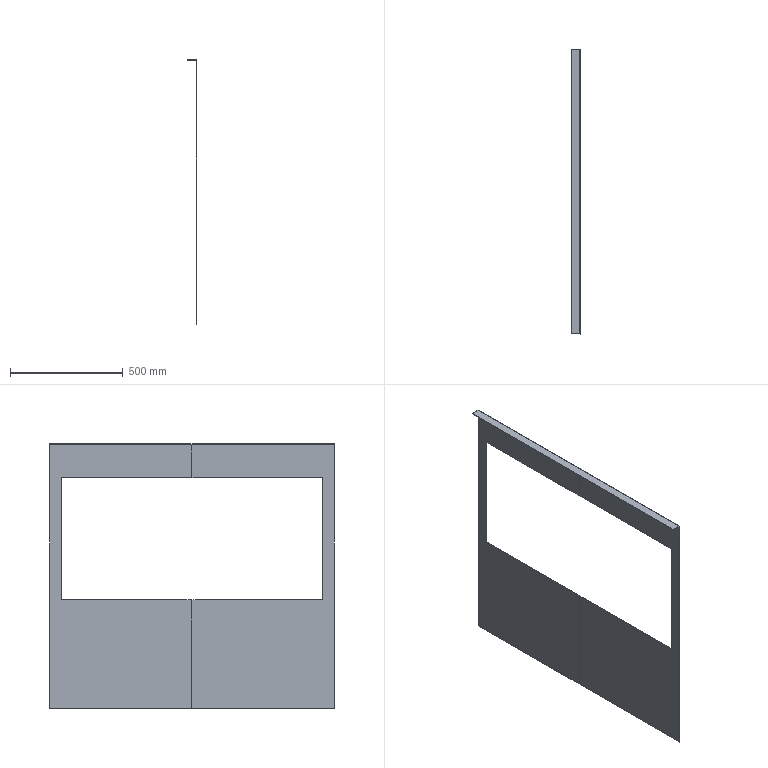Part | NX | features BREP 1 | 1 solid | 23 faces | box 42 x 1258 x 1171 mm | volume 1789977 mm3 | plane 20 | cylinder 3 | commonest cylinder face diameters 6 x2 10 x1
STEP:
#1=CARTESIAN_POINT('',(2104.579,0.000000001,74.));
#2=VERTEX_POINT('',#1);
#3=CARTESIAN_POINT('',(2104.579,0.,553.577));
#4=VERTEX_POINT('',#3);
#5=CARTESIAN_POINT('',(2104.579,-0.000000001,313.789));
#6=DIRECTION('',(0.,0.,1.));
#7=VECTOR('',#6,1000.);
#8=LINE('',#5,#7);
#9=EDGE_CURVE('',#2,#4,#8,.T.);
#10=ORIENTED_EDGE('',*,*,#9,.F.);
#11=CARTESIAN_POINT('',(2104.579,-629.17,74.));
#12=VERTEX_POINT('',#11);
#13=CARTESIAN_POINT('',(2104.579,-314.585,74.));
#14=DIRECTION('',(0.,-1.,0.));
#15=VECTOR('',#14,1000.);
#16=LINE('',#13,#15);
#17=EDGE_CURVE('',#2,#12,#16,.T.);
#18=ORIENTED_EDGE('',*,*,#17,.T.);
#19=CARTESIAN_POINT('',(2104.579,-629.17,1239.934));
#20=VERTEX_POINT('',#19);
#21=CARTESIAN_POINT('',(2104.579,-629.17,656.967));
#22=DIRECTION('',(0.,0.,1.));
#23=VECTOR('',#22,1000.);
#24=LINE('',#21,#23);
#25=EDGE_CURVE('',#12,#20,#24,.T.);
#26=ORIENTED_EDGE('',*,*,#25,.T.);
#27=CARTESIAN_POINT('',(2104.579,0.,1239.934));
#28=VERTEX_POINT('',#27);
#29=CARTESIAN_POINT('',(2104.579,0.,1239.934));
#30=DIRECTION('',(0.,-1.,0.));
#31=VECTOR('',#30,1000.);
#32=LINE('',#29,#31);
#33=EDGE_CURVE('',#28,#20,#32,.T.);
#34=ORIENTED_EDGE('',*,*,#33,.F.);
#35=CARTESIAN_POINT('',(2104.579,0.000000001,1094.538));
#36=VERTEX_POINT('',#35);
#37=CARTESIAN_POINT('',(2104.579,-0.000000001,1167.236));
#38=DIRECTION('',(0.,0.,1.));
#39=VECTOR('',#38,1000.);
#40=LINE('',#37,#39);
#41=EDGE_CURVE('',#36,#28,#40,.T.);
#42=ORIENTED_EDGE('',*,*,#41,.F.);
#43=CARTESIAN_POINT('',(2104.579,-579.171,1094.538));
#44=VERTEX_POINT('',#43);
#45=CARTESIAN_POINT('',(2104.579,-289.585,1094.538));
#46=DIRECTION('',(0.,-1.,0.));
#47=VECTOR('',#46,1000.);
#48=LINE('',#45,#47);
#49=EDGE_CURVE('',#36,#44,#48,.T.);
#50=ORIENTED_EDGE('',*,*,#49,.T.);
#51=CARTESIAN_POINT('',(2104.579,-579.171,553.577));
#52=VERTEX_POINT('',#51);
#53=CARTESIAN_POINT('',(2104.579,-579.171,824.058));
#54=DIRECTION('',(0.,0.,1.));
#55=VECTOR('',#54,1000.);
#56=LINE('',#53,#55);
#57=EDGE_CURVE('',#52,#44,#56,.T.);
#58=ORIENTED_EDGE('',*,*,#57,.F.);
#59=CARTESIAN_POINT('',(2104.579,-21.22,553.577));
#60=VERTEX_POINT('',#59);
#61=CARTESIAN_POINT('',(2104.579,-300.195,553.577));
#62=DIRECTION('',(0.,-1.,0.));
#63=VECTOR('',#62,1000.);
#64=LINE('',#61,#63);
#65=EDGE_CURVE('',#52,#60,#64,.F.);
#66=ORIENTED_EDGE('',*,*,#65,.T.);
#67=CARTESIAN_POINT('',(2104.579,-8.78,553.577));
#68=VERTEX_POINT('',#67);
#69=CARTESIAN_POINT('',(2104.579,-15.,553.577));
#70=DIRECTION('',(0.,-1.,0.));
#71=VECTOR('',#70,1000.);
#72=LINE('',#69,#71);
#73=EDGE_CURVE('',#68,#60,#72,.T.);
#74=ORIENTED_EDGE('',*,*,#73,.F.);
#75=CARTESIAN_POINT('',(2104.579,-4.39,553.577));
#76=DIRECTION('',(0.,1.,0.));
#77=VECTOR('',#76,1000.);
#78=LINE('',#75,#77);
#79=EDGE_CURVE('',#4,#68,#78,.F.);
#80=ORIENTED_EDGE('',*,*,#79,.F.);
#81=EDGE_LOOP('',(#10,#18,#26,#34,#42,#50,#58,#66,#74,#80));
#82=FACE_BOUND('',#81,.T.);
#83=CARTESIAN_POINT('',(2104.579,0.,74.));
#84=DIRECTION('',(-1.,0.,0.));
#85=DIRECTION('',(0.,-1.,0.));
#86=AXIS2_PLACEMENT_3D('',#83,#84,#85);
#87=PLANE('',#86);
#88=ADVANCED_FACE('',(#82),#87,.T.);
#89=CARTESIAN_POINT('',(2104.579,8.78,553.577));
#90=VERTEX_POINT('',#89);
#91=CARTESIAN_POINT('',(2104.579,4.39,553.577));
#92=DIRECTION('',(0.,1.,0.));
#93=VECTOR('',#92,1000.);
#94=LINE('',#91,#93);
#95=EDGE_CURVE('',#4,#90,#94,.T.);
#96=ORIENTED_EDGE('',*,*,#95,.T.);
#97=CARTESIAN_POINT('',(2104.579,579.171,553.577));
#98=VERTEX_POINT('',#97);
#99=CARTESIAN_POINT('',(2104.579,293.975,553.577));
#100=DIRECTION('',(0.,1.,0.));
#101=VECTOR('',#100,1000.);
#102=LINE('',#99,#101);
#103=EDGE_CURVE('',#90,#98,#102,.T.);
#104=ORIENTED_EDGE('',*,*,#103,.T.);
#105=CARTESIAN_POINT('',(2104.579,579.171,1094.538));
#106=VERTEX_POINT('',#105);
#107=CARTESIAN_POINT('',(2104.579,579.171,824.058));
#108=DIRECTION('',(0.,0.,1.));
#109=VECTOR('',#108,1000.);
#110=LINE('',#107,#109);
#111=EDGE_CURVE('',#98,#106,#110,.T.);
#112=ORIENTED_EDGE('',*,*,#111,.T.);
#113=CARTESIAN_POINT('',(2104.579,289.585,1094.538));
#114=DIRECTION('',(0.,1.,0.));
#115=VECTOR('',#114,1000.);
#116=LINE('',#113,#115);
#117=EDGE_CURVE('',#36,#106,#116,.T.);
#118=ORIENTED_EDGE('',*,*,#117,.F.);
#119=ORIENTED_EDGE('',*,*,#41,.T.);
#120=CARTESIAN_POINT('',(2104.579,629.17,1239.934));
#121=VERTEX_POINT('',#120);
#122=CARTESIAN_POINT('',(2104.579,0.,1239.934));
#123=DIRECTION('',(0.,-1.,0.));
#124=VECTOR('',#123,1000.);
#125=LINE('',#122,#124);
#126=EDGE_CURVE('',#121,#28,#125,.T.);
#127=ORIENTED_EDGE('',*,*,#126,.F.);
#128=CARTESIAN_POINT('',(2104.579,629.17,74.));
#129=VERTEX_POINT('',#128);
#130=CARTESIAN_POINT('',(2104.579,629.17,656.967));
#131=DIRECTION('',(0.,0.,1.));
#132=VECTOR('',#131,1000.);
#133=LINE('',#130,#132);
#134=EDGE_CURVE('',#129,#121,#133,.T.);
#135=ORIENTED_EDGE('',*,*,#134,.F.);
#136=CARTESIAN_POINT('',(2104.579,314.585,74.));
#137=DIRECTION('',(0.,1.,0.));
#138=VECTOR('',#137,1000.);
#139=LINE('',#136,#138);
#140=EDGE_CURVE('',#2,#129,#139,.T.);
#141=ORIENTED_EDGE('',*,*,#140,.F.);
#142=ORIENTED_EDGE('',*,*,#9,.T.);
#143=EDGE_LOOP('',(#96,#104,#112,#118,#119,#127,#135,#141,#142));
#144=FACE_BOUND('',#143,.T.);
#145=CARTESIAN_POINT('',(2104.579,0.,74.));
#146=DIRECTION('',(1.,0.,0.));
#147=DIRECTION('',(0.,1.,0.));
#148=AXIS2_PLACEMENT_3D('',#145,#146,#147);
#149=PLANE('',#148);
#150=ADVANCED_FACE('',(#144),#149,.F.);
#151=CARTESIAN_POINT('',(2106.579,579.171,553.577));
#152=VERTEX_POINT('',#151);
#153=CARTESIAN_POINT('',(2106.579,579.171,1094.538));
#154=VERTEX_POINT('',#153);
#155=CARTESIAN_POINT('',(2106.579,579.171,824.058));
#156=DIRECTION('',(0.,0.,1.));
#157=VECTOR('',#156,1000.);
#158=LINE('',#155,#157);
#159=EDGE_CURVE('',#152,#154,#158,.T.);
#160=ORIENTED_EDGE('',*,*,#159,.T.);
#161=CARTESIAN_POINT('',(2105.579,579.171,1094.538));
#162=DIRECTION('',(1.,-0.000000002,0.));
#163=VECTOR('',#162,1000.);
#164=LINE('',#161,#163);
#165=EDGE_CURVE('',#106,#154,#164,.T.);
#166=ORIENTED_EDGE('',*,*,#165,.F.);
#167=ORIENTED_EDGE('',*,*,#111,.F.);
#168=CARTESIAN_POINT('',(2105.579,579.171,553.577));
#169=DIRECTION('',(1.,0.,0.));
#170=VECTOR('',#169,1000.);
#171=LINE('',#168,#170);
#172=EDGE_CURVE('',#98,#152,#171,.T.);
#173=ORIENTED_EDGE('',*,*,#172,.T.);
#174=EDGE_LOOP('',(#160,#166,#167,#173));
#175=FACE_BOUND('',#174,.T.);
#176=CARTESIAN_POINT('',(2106.579,579.171,553.577));
#177=DIRECTION('',(0.,1.,0.));
#178=DIRECTION('',(0.,0.,1.));
#179=AXIS2_PLACEMENT_3D('',#176,#177,#178);
#180=PLANE('',#179);
#181=ADVANCED_FACE('',(#175),#180,.F.);
#182=CARTESIAN_POINT('',(2106.579,0.,1094.538));
#183=VERTEX_POINT('',#182);
#184=CARTESIAN_POINT('',(2106.579,289.585,1094.538));
#185=DIRECTION('',(0.,1.,0.));
#186=VECTOR('',#185,1000.);
#187=LINE('',#184,#186);
#188=EDGE_CURVE('',#183,#154,#187,.T.);
#189=ORIENTED_EDGE('',*,*,#188,.F.);
#190=CARTESIAN_POINT('',(2105.579,0.,1094.538));
#191=DIRECTION('',(-1.,0.,0.));
#192=VECTOR('',#191,1000.);
#193=LINE('',#190,#192);
#194=EDGE_CURVE('',#183,#36,#193,.T.);
#195=ORIENTED_EDGE('',*,*,#194,.T.);
#196=ORIENTED_EDGE('',*,*,#117,.T.);
#197=ORIENTED_EDGE('',*,*,#165,.T.);
#198=EDGE_LOOP('',(#189,#195,#196,#197));
#199=FACE_BOUND('',#198,.T.);
#200=CARTESIAN_POINT('',(2106.579,579.171,1094.538));
#201=DIRECTION('',(0.,0.,1.));
#202=DIRECTION('',(0.,-1.,0.));
#203=AXIS2_PLACEMENT_3D('',#200,#201,#202);
#204=PLANE('',#203);
#205=ADVANCED_FACE('',(#199),#204,.F.);
#206=CARTESIAN_POINT('',(2106.579,0.,74.));
#207=VERTEX_POINT('',#206);
#208=CARTESIAN_POINT('',(2106.579,629.17,74.));
#209=VERTEX_POINT('',#208);
#210=CARTESIAN_POINT('',(2106.579,314.585,74.));
#211=DIRECTION('',(0.,1.,0.));
#212=VECTOR('',#211,1000.);
#213=LINE('',#210,#212);
#214=EDGE_CURVE('',#207,#209,#213,.T.);
#215=ORIENTED_EDGE('',*,*,#214,.F.);
#216=CARTESIAN_POINT('',(2105.579,0.,74.));
#217=DIRECTION('',(-1.,0.,0.));
#218=VECTOR('',#217,1000.);
#219=LINE('',#216,#218);
#220=EDGE_CURVE('',#207,#2,#219,.T.);
#221=ORIENTED_EDGE('',*,*,#220,.T.);
#222=ORIENTED_EDGE('',*,*,#140,.T.);
#223=CARTESIAN_POINT('',(2105.579,629.17,74.));
#224=DIRECTION('',(1.,0.,0.));
#225=VECTOR('',#224,1000.);
#226=LINE('',#223,#225);
#227=EDGE_CURVE('',#129,#209,#226,.T.);
#228=ORIENTED_EDGE('',*,*,#227,.T.);
#229=EDGE_LOOP('',(#215,#221,#222,#228));
#230=FACE_BOUND('',#229,.T.);
#231=CARTESIAN_POINT('',(2106.579,314.585,74.));
#232=DIRECTION('',(0.,0.,-1.));
#233=DIRECTION('',(1.,0.,0.));
#234=AXIS2_PLACEMENT_3D('',#231,#232,#233);
#235=PLANE('',#234);
#236=ADVANCED_FACE('',(#230),#235,.T.);
#237=CARTESIAN_POINT('',(2106.579,-629.17,74.));
#238=VERTEX_POINT('',#237);
#239=CARTESIAN_POINT('',(2105.579,-629.17,74.));
#240=DIRECTION('',(-1.,0.,0.));
#241=VECTOR('',#240,1000.);
#242=LINE('',#239,#241);
#243=EDGE_CURVE('',#238,#12,#242,.T.);
#244=ORIENTED_EDGE('',*,*,#243,.T.);
#245=ORIENTED_EDGE('',*,*,#17,.F.);
#246=ORIENTED_EDGE('',*,*,#220,.F.);
#247=CARTESIAN_POINT('',(2106.579,-314.585,74.));
#248=DIRECTION('',(0.,-1.,0.));
#249=VECTOR('',#248,1000.);
#250=LINE('',#247,#249);
#251=EDGE_CURVE('',#207,#238,#250,.T.);
#252=ORIENTED_EDGE('',*,*,#251,.T.);
#253=EDGE_LOOP('',(#244,#245,#246,#252));
#254=FACE_BOUND('',#253,.T.);
#255=CARTESIAN_POINT('',(2106.579,0.,74.));
#256=DIRECTION('',(0.,0.,-1.));
#257=DIRECTION('',(0.,-1.,0.));
#258=AXIS2_PLACEMENT_3D('',#255,#256,#257);
#259=PLANE('',#258);
#260=ADVANCED_FACE('',(#254),#259,.T.);
#261=CARTESIAN_POINT('',(2106.579,-579.171,1094.538));
#262=VERTEX_POINT('',#261);
#263=CARTESIAN_POINT('',(2105.579,-579.171,1094.538));
#264=DIRECTION('',(-1.,0.,0.));
#265=VECTOR('',#264,1000.);
#266=LINE('',#263,#265);
#267=EDGE_CURVE('',#262,#44,#266,.T.);
#268=ORIENTED_EDGE('',*,*,#267,.T.);
#269=ORIENTED_EDGE('',*,*,#49,.F.);
#270=ORIENTED_EDGE('',*,*,#194,.F.);
#271=CARTESIAN_POINT('',(2106.579,-289.585,1094.538));
#272=DIRECTION('',(0.,-1.,0.));
#273=VECTOR('',#272,1000.);
#274=LINE('',#271,#273);
#275=EDGE_CURVE('',#183,#262,#274,.T.);
#276=ORIENTED_EDGE('',*,*,#275,.T.);
#277=EDGE_LOOP('',(#268,#269,#270,#276));
#278=FACE_BOUND('',#277,.T.);
#279=CARTESIAN_POINT('',(2106.579,-579.171,1094.538));
#280=DIRECTION('',(0.,0.,1.));
#281=DIRECTION('',(0.,1.,0.));
#282=AXIS2_PLACEMENT_3D('',#279,#280,#281);
#283=PLANE('',#282);
#284=ADVANCED_FACE('',(#278),#283,.F.);
#285=CARTESIAN_POINT('',(2106.579,-579.171,553.577));
#286=VERTEX_POINT('',#285);
#287=CARTESIAN_POINT('',(2105.579,-579.171,553.577));
#288=DIRECTION('',(-1.,0.,0.));
#289=VECTOR('',#288,1000.);
#290=LINE('',#287,#289);
#291=EDGE_CURVE('',#286,#52,#290,.T.);
#292=ORIENTED_EDGE('',*,*,#291,.T.);
#293=ORIENTED_EDGE('',*,*,#57,.T.);
#294=ORIENTED_EDGE('',*,*,#267,.F.);
#295=CARTESIAN_POINT('',(2106.579,-579.171,824.058));
#296=DIRECTION('',(0.,0.,1.));
#297=VECTOR('',#296,1000.);
#298=LINE('',#295,#297);
#299=EDGE_CURVE('',#286,#262,#298,.T.);
#300=ORIENTED_EDGE('',*,*,#299,.F.);
#301=EDGE_LOOP('',(#292,#293,#294,#300));
#302=FACE_BOUND('',#301,.T.);
#303=CARTESIAN_POINT('',(2106.579,-579.171,553.577));
#304=DIRECTION('',(0.,-1.,0.));
#305=DIRECTION('',(0.,0.,1.));
#306=AXIS2_PLACEMENT_3D('',#303,#304,#305);
#307=PLANE('',#306);
#308=ADVANCED_FACE('',(#302),#307,.F.);
#309=ORIENTED_EDGE('',*,*,#73,.T.);
#310=ORIENTED_EDGE('',*,*,#65,.F.);
#311=ORIENTED_EDGE('',*,*,#291,.F.);
#312=CARTESIAN_POINT('',(2106.579,-21.22,553.577));
#313=VERTEX_POINT('',#312);
#314=CARTESIAN_POINT('',(2106.579,-300.195,553.577));
#315=DIRECTION('',(0.,-1.,0.));
#316=VECTOR('',#315,1000.);
#317=LINE('',#314,#316);
#318=EDGE_CURVE('',#313,#286,#317,.T.);
#319=ORIENTED_EDGE('',*,*,#318,.F.);
#320=CARTESIAN_POINT('',(2106.579,-8.78,553.577));
#321=VERTEX_POINT('',#320);
#322=CARTESIAN_POINT('',(2106.579,-15.,553.577));
#323=DIRECTION('',(0.,-1.,0.));
#324=VECTOR('',#323,1000.);
#325=LINE('',#322,#324);
#326=EDGE_CURVE('',#321,#313,#325,.T.);
#327=ORIENTED_EDGE('',*,*,#326,.F.);
#328=CARTESIAN_POINT('',(2106.579,0.,553.577));
#329=VERTEX_POINT('',#328);
#330=CARTESIAN_POINT('',(2106.579,-4.39,553.577));
#331=DIRECTION('',(0.,-1.,0.));
#332=VECTOR('',#331,1000.);
#333=LINE('',#330,#332);
#334=EDGE_CURVE('',#329,#321,#333,.T.);
#335=ORIENTED_EDGE('',*,*,#334,.F.);
#336=CARTESIAN_POINT('',(2106.579,8.78,553.577));
#337=VERTEX_POINT('',#336);
#338=CARTESIAN_POINT('',(2106.579,4.39,553.577));
#339=DIRECTION('',(0.,1.,0.));
#340=VECTOR('',#339,1000.);
#341=LINE('',#338,#340);
#342=EDGE_CURVE('',#329,#337,#341,.T.);
#343=ORIENTED_EDGE('',*,*,#342,.T.);
#344=CARTESIAN_POINT('',(2106.579,293.975,553.577));
#345=DIRECTION('',(0.,1.,0.));
#346=VECTOR('',#345,1000.);
#347=LINE('',#344,#346);
#348=EDGE_CURVE('',#337,#152,#347,.T.);
#349=ORIENTED_EDGE('',*,*,#348,.T.);
#350=ORIENTED_EDGE('',*,*,#172,.F.);
#351=ORIENTED_EDGE('',*,*,#103,.F.);
#352=ORIENTED_EDGE('',*,*,#95,.F.);
#353=ORIENTED_EDGE('',*,*,#79,.T.);
#354=EDGE_LOOP('',(#309,#310,#311,#319,#327,#335,#343,#349,#350,#351,#352,#353));
#355=FACE_BOUND('',#354,.T.);
#356=CARTESIAN_POINT('',(2106.579,8.78,553.577));
#357=DIRECTION('',(0.,0.,-1.));
#358=DIRECTION('',(0.,1.,0.));
#359=AXIS2_PLACEMENT_3D('',#356,#357,#358);
#360=PLANE('',#359);
#361=ADVANCED_FACE('',(#355),#360,.F.);
#362=CARTESIAN_POINT('',(2106.579,-629.17,1239.934));
#363=VERTEX_POINT('',#362);
#364=CARTESIAN_POINT('',(2105.579,-629.17,1239.934));
#365=DIRECTION('',(1.,0.,0.));
#366=VECTOR('',#365,1000.);
#367=LINE('',#364,#366);
#368=EDGE_CURVE('',#20,#363,#367,.T.);
#369=ORIENTED_EDGE('',*,*,#368,.F.);
#370=ORIENTED_EDGE('',*,*,#25,.F.);
#371=ORIENTED_EDGE('',*,*,#243,.F.);
#372=CARTESIAN_POINT('',(2106.579,-629.17,656.967));
#373=DIRECTION('',(0.,0.,1.));
#374=VECTOR('',#373,1000.);
#375=LINE('',#372,#374);
#376=EDGE_CURVE('',#238,#363,#375,.T.);
#377=ORIENTED_EDGE('',*,*,#376,.T.);
#378=EDGE_LOOP('',(#369,#370,#371,#377));
#379=FACE_BOUND('',#378,.T.);
#380=CARTESIAN_POINT('',(2106.579,-629.17,74.));
#381=DIRECTION('',(0.,-1.,0.));
#382=DIRECTION('',(0.,0.,1.));
#383=AXIS2_PLACEMENT_3D('',#380,#381,#382);
#384=PLANE('',#383);
#385=ADVANCED_FACE('',(#379),#384,.T.);
#386=CARTESIAN_POINT('',(2103.7,629.17,1242.055));
#387=VERTEX_POINT('',#386);
#388=CARTESIAN_POINT('',(2101.579,629.17,1239.934));
#389=DIRECTION('',(0.,-1.,0.));
#390=DIRECTION('',(1.,0.,0.));
#391=AXIS2_PLACEMENT_3D('',#388,#389,#390);
#392=CIRCLE('',#391,3.);
#393=EDGE_CURVE('',#121,#387,#392,.T.);
#394=ORIENTED_EDGE('',*,*,#393,.F.);
#395=ORIENTED_EDGE('',*,*,#126,.T.);
#396=ORIENTED_EDGE('',*,*,#33,.T.);
#397=CARTESIAN_POINT('',(2103.7,-629.17,1242.055));
#398=VERTEX_POINT('',#397);
#399=CARTESIAN_POINT('',(2101.579,-629.17,1239.934));
#400=DIRECTION('',(0.,-1.,0.));
#401=DIRECTION('',(1.,0.,0.));
#402=AXIS2_PLACEMENT_3D('',#399,#400,#401);
#403=CIRCLE('',#402,3.);
#404=EDGE_CURVE('',#20,#398,#403,.T.);
#405=ORIENTED_EDGE('',*,*,#404,.T.);
#406=CARTESIAN_POINT('',(2103.7,0.,1242.055));
#407=DIRECTION('',(0.,-1.,0.));
#408=VECTOR('',#407,1000.);
#409=LINE('',#406,#408);
#410=EDGE_CURVE('',#387,#398,#409,.T.);
#411=ORIENTED_EDGE('',*,*,#410,.F.);
#412=EDGE_LOOP('',(#394,#395,#396,#405,#411));
#413=FACE_BOUND('',#412,.T.);
#414=CARTESIAN_POINT('',(2101.579,0.,1239.934));
#415=DIRECTION('',(0.,-1.,0.));
#416=DIRECTION('',(-0.7071,0.,-0.7071));
#417=AXIS2_PLACEMENT_3D('',#414,#415,#416);
#418=CYLINDRICAL_SURFACE('',#417,3.);
#419=ADVANCED_FACE('',(#413),#418,.F.);
#420=CARTESIAN_POINT('',(2106.579,629.17,1239.934));
#421=VERTEX_POINT('',#420);
#422=CARTESIAN_POINT('',(2106.579,629.17,656.967));
#423=DIRECTION('',(0.,0.,1.));
#424=VECTOR('',#423,1000.);
#425=LINE('',#422,#424);
#426=EDGE_CURVE('',#209,#421,#425,.T.);
#427=ORIENTED_EDGE('',*,*,#426,.F.);
#428=ORIENTED_EDGE('',*,*,#227,.F.);
#429=ORIENTED_EDGE('',*,*,#134,.T.);
#430=CARTESIAN_POINT('',(2105.579,629.17,1239.934));
#431=DIRECTION('',(1.,0.,0.));
#432=VECTOR('',#431,1000.);
#433=LINE('',#430,#432);
#434=EDGE_CURVE('',#121,#421,#433,.T.);
#435=ORIENTED_EDGE('',*,*,#434,.T.);
#436=EDGE_LOOP('',(#427,#428,#429,#435));
#437=FACE_BOUND('',#436,.T.);
#438=CARTESIAN_POINT('',(2106.579,629.17,74.));
#439=DIRECTION('',(0.,1.,0.));
#440=DIRECTION('',(0.,0.,1.));
#441=AXIS2_PLACEMENT_3D('',#438,#439,#440);
#442=PLANE('',#441);
#443=ADVANCED_FACE('',(#437),#442,.T.);
#444=CARTESIAN_POINT('',(2106.579,0.,313.789));
#445=DIRECTION('',(0.,0.,1.));
#446=VECTOR('',#445,1000.);
#447=LINE('',#444,#446);
#448=EDGE_CURVE('',#207,#329,#447,.T.);
#449=ORIENTED_EDGE('',*,*,#448,.F.);
#450=ORIENTED_EDGE('',*,*,#214,.T.);
#451=ORIENTED_EDGE('',*,*,#426,.T.);
#452=CARTESIAN_POINT('',(2106.579,0.,1239.934));
#453=VERTEX_POINT('',#452);
#454=CARTESIAN_POINT('',(2106.579,0.,1239.934));
#455=DIRECTION('',(0.,-1.,0.));
#456=VECTOR('',#455,1000.);
#457=LINE('',#454,#456);
#458=EDGE_CURVE('',#421,#453,#457,.T.);
#459=ORIENTED_EDGE('',*,*,#458,.T.);
#460=CARTESIAN_POINT('',(2106.579,0.,1167.236));
#461=DIRECTION('',(0.,0.,1.));
#462=VECTOR('',#461,1000.);
#463=LINE('',#460,#462);
#464=EDGE_CURVE('',#183,#453,#463,.T.);
#465=ORIENTED_EDGE('',*,*,#464,.F.);
#466=ORIENTED_EDGE('',*,*,#188,.T.);
#467=ORIENTED_EDGE('',*,*,#159,.F.);
#468=ORIENTED_EDGE('',*,*,#348,.F.);
#469=ORIENTED_EDGE('',*,*,#342,.F.);
#470=EDGE_LOOP('',(#449,#450,#451,#459,#465,#466,#467,#468,#469));
#471=FACE_BOUND('',#470,.T.);
#472=CARTESIAN_POINT('',(2106.579,-7.184,67.));
#473=DIRECTION('',(1.,0.,0.));
#474=DIRECTION('',(0.,1.,0.));
#475=AXIS2_PLACEMENT_3D('',#472,#473,#474);
#476=PLANE('',#475);
#477=ADVANCED_FACE('',(#471),#476,.T.);
#478=ORIENTED_EDGE('',*,*,#334,.T.);
#479=ORIENTED_EDGE('',*,*,#326,.T.);
#480=ORIENTED_EDGE('',*,*,#318,.T.);
#481=ORIENTED_EDGE('',*,*,#299,.T.);
#482=ORIENTED_EDGE('',*,*,#275,.F.);
#483=ORIENTED_EDGE('',*,*,#464,.T.);
#484=CARTESIAN_POINT('',(2106.579,0.,1239.934));
#485=DIRECTION('',(0.,-1.,0.));
#486=VECTOR('',#485,1000.);
#487=LINE('',#484,#486);
#488=EDGE_CURVE('',#453,#363,#487,.T.);
#489=ORIENTED_EDGE('',*,*,#488,.T.);
#490=ORIENTED_EDGE('',*,*,#376,.F.);
#491=ORIENTED_EDGE('',*,*,#251,.F.);
#492=ORIENTED_EDGE('',*,*,#448,.T.);
#493=EDGE_LOOP('',(#478,#479,#480,#481,#482,#483,#489,#490,#491,#492));
#494=FACE_BOUND('',#493,.T.);
#495=CARTESIAN_POINT('',(2106.579,7.184,67.));
#496=DIRECTION('',(-1.,0.,0.));
#497=DIRECTION('',(0.,-1.,0.));
#498=AXIS2_PLACEMENT_3D('',#495,#496,#497);
#499=PLANE('',#498);
#500=ADVANCED_FACE('',(#494),#499,.F.);
#501=CARTESIAN_POINT('',(2101.579,-629.17,1242.934));
#502=VERTEX_POINT('',#501);
#503=CARTESIAN_POINT('',(2101.579,-629.17,1244.934));
#504=VERTEX_POINT('',#503);
#505=CARTESIAN_POINT('',(2101.579,-629.17,1243.934));
#506=DIRECTION('',(0.,0.,1.));
#507=VECTOR('',#506,1000.);
#508=LINE('',#505,#507);
#509=EDGE_CURVE('',#502,#504,#508,.T.);
#510=ORIENTED_EDGE('',*,*,#509,.F.);
#511=CARTESIAN_POINT('',(2101.579,-629.17,1239.934));
#512=DIRECTION('',(0.,-1.,0.));
#513=DIRECTION('',(1.,0.,0.));
#514=AXIS2_PLACEMENT_3D('',#511,#512,#513);
#515=CIRCLE('',#514,3.);
#516=EDGE_CURVE('',#398,#502,#515,.T.);
#517=ORIENTED_EDGE('',*,*,#516,.F.);
#518=ORIENTED_EDGE('',*,*,#404,.F.);
#519=ORIENTED_EDGE('',*,*,#368,.T.);
#520=CARTESIAN_POINT('',(2101.579,-629.17,1239.934));
#521=DIRECTION('',(0.,-1.,0.));
#522=DIRECTION('',(1.,0.,0.));
#523=AXIS2_PLACEMENT_3D('',#520,#521,#522);
#524=CIRCLE('',#523,5.);
#525=EDGE_CURVE('',#363,#504,#524,.T.);
#526=ORIENTED_EDGE('',*,*,#525,.T.);
#527=EDGE_LOOP('',(#510,#517,#518,#519,#526));
#528=FACE_BOUND('',#527,.T.);
#529=CARTESIAN_POINT('',(2106.579,-629.17,1239.934));
#530=DIRECTION('',(0.,-1.,0.));
#531=DIRECTION('',(-0.3827,0.,0.9239));
#532=AXIS2_PLACEMENT_3D('',#529,#530,#531);
#533=PLANE('',#532);
#534=ADVANCED_FACE('',(#528),#533,.T.);
#535=ORIENTED_EDGE('',*,*,#516,.T.);
#536=CARTESIAN_POINT('',(2101.579,629.17,1242.934));
#537=VERTEX_POINT('',#536);
#538=CARTESIAN_POINT('',(2101.579,0.,1242.934));
#539=DIRECTION('',(0.,-1.,0.));
#540=VECTOR('',#539,1000.);
#541=LINE('',#538,#540);
#542=EDGE_CURVE('',#537,#502,#541,.T.);
#543=ORIENTED_EDGE('',*,*,#542,.F.);
#544=CARTESIAN_POINT('',(2101.579,629.17,1239.934));
#545=DIRECTION('',(0.,-1.,0.));
#546=DIRECTION('',(1.,0.,0.));
#547=AXIS2_PLACEMENT_3D('',#544,#545,#546);
#548=CIRCLE('',#547,3.);
#549=EDGE_CURVE('',#387,#537,#548,.T.);
#550=ORIENTED_EDGE('',*,*,#549,.F.);
#551=ORIENTED_EDGE('',*,*,#410,.T.);
#552=EDGE_LOOP('',(#535,#543,#550,#551));
#553=FACE_BOUND('',#552,.T.);
#554=CARTESIAN_POINT('',(2101.579,0.,1239.934));
#555=DIRECTION('',(0.,-1.,0.));
#556=DIRECTION('',(0.7071,0.,0.7071));
#557=AXIS2_PLACEMENT_3D('',#554,#555,#556);
#558=CYLINDRICAL_SURFACE('',#557,3.);
#559=ADVANCED_FACE('',(#553),#558,.F.);
#560=CARTESIAN_POINT('',(2101.579,629.17,1244.934));
#561=VERTEX_POINT('',#560);
#562=CARTESIAN_POINT('',(2101.579,629.17,1239.934));
#563=DIRECTION('',(0.,-1.,0.));
#564=DIRECTION('',(1.,0.,0.));
#565=AXIS2_PLACEMENT_3D('',#562,#563,#564);
#566=CIRCLE('',#565,5.);
#567=EDGE_CURVE('',#421,#561,#566,.T.);
#568=ORIENTED_EDGE('',*,*,#567,.F.);
#569=ORIENTED_EDGE('',*,*,#434,.F.);
#570=ORIENTED_EDGE('',*,*,#393,.T.);
#571=ORIENTED_EDGE('',*,*,#549,.T.);
#572=CARTESIAN_POINT('',(2101.579,629.17,1243.934));
#573=DIRECTION('',(0.,0.,1.));
#574=VECTOR('',#573,1000.);
#575=LINE('',#572,#574);
#576=EDGE_CURVE('',#537,#561,#575,.T.);
#577=ORIENTED_EDGE('',*,*,#576,.T.);
#578=EDGE_LOOP('',(#568,#569,#570,#571,#577));
#579=FACE_BOUND('',#578,.T.);
#580=CARTESIAN_POINT('',(2106.579,629.17,1239.934));
#581=DIRECTION('',(0.,-1.,0.));
#582=DIRECTION('',(-0.3827,0.,0.9239));
#583=AXIS2_PLACEMENT_3D('',#580,#581,#582);
#584=PLANE('',#583);
#585=ADVANCED_FACE('',(#579),#584,.F.);
#586=CARTESIAN_POINT('',(2101.579,0.,1244.934));
#587=DIRECTION('',(0.,1.,0.));
#588=VECTOR('',#587,1000.);
#589=LINE('',#586,#588);
#590=EDGE_CURVE('',#504,#561,#589,.T.);
#591=ORIENTED_EDGE('',*,*,#590,.F.);
#592=ORIENTED_EDGE('',*,*,#525,.F.);
#593=ORIENTED_EDGE('',*,*,#488,.F.);
#594=ORIENTED_EDGE('',*,*,#458,.F.);
#595=ORIENTED_EDGE('',*,*,#567,.T.);
#596=EDGE_LOOP('',(#591,#592,#593,#594,#595));
#597=FACE_BOUND('',#596,.T.);
#598=CARTESIAN_POINT('',(2101.579,0.,1239.934));
#599=DIRECTION('',(0.,-1.,0.));
#600=DIRECTION('',(1.,0.,0.));
#601=AXIS2_PLACEMENT_3D('',#598,#599,#600);
#602=CYLINDRICAL_SURFACE('',#601,5.);
#603=ADVANCED_FACE('',(#597),#602,.T.);
#604=CARTESIAN_POINT('',(2064.579,-629.17,1244.934));
#605=VERTEX_POINT('',#604);
#606=CARTESIAN_POINT('',(2083.079,-629.17,1244.934));
#607=DIRECTION('',(1.,0.,0.));
#608=VECTOR('',#607,1000.);
#609=LINE('',#606,#608);
#610=EDGE_CURVE('',#605,#504,#609,.T.);
#611=ORIENTED_EDGE('',*,*,#610,.F.);
#612=CARTESIAN_POINT('',(2064.579,-629.17,1242.934));
#613=VERTEX_POINT('',#612);
#614=CARTESIAN_POINT('',(2064.579,-629.17,1243.934));
#615=DIRECTION('',(0.,0.,1.));
#616=VECTOR('',#615,1000.);
#617=LINE('',#614,#616);
#618=EDGE_CURVE('',#613,#605,#617,.T.);
#619=ORIENTED_EDGE('',*,*,#618,.F.);
#620=CARTESIAN_POINT('',(2083.079,-629.17,1242.934));
#621=DIRECTION('',(1.,0.,0.));
#622=VECTOR('',#621,1000.);
#623=LINE('',#620,#622);
#624=EDGE_CURVE('',#613,#502,#623,.T.);
#625=ORIENTED_EDGE('',*,*,#624,.T.);
#626=ORIENTED_EDGE('',*,*,#509,.T.);
#627=EDGE_LOOP('',(#611,#619,#625,#626));
#628=FACE_BOUND('',#627,.T.);
#629=CARTESIAN_POINT('',(2083.079,-629.17,1244.934));
#630=DIRECTION('',(0.,1.,0.));
#631=DIRECTION('',(1.,0.,0.));
#632=AXIS2_PLACEMENT_3D('',#629,#630,#631);
#633=PLANE('',#632);
#634=ADVANCED_FACE('',(#628),#633,.F.);
#635=ORIENTED_EDGE('',*,*,#624,.F.);
#636=CARTESIAN_POINT('',(2064.579,629.17,1242.934));
#637=VERTEX_POINT('',#636);
#638=CARTESIAN_POINT('',(2064.579,0.,1242.934));
#639=DIRECTION('',(0.,1.,0.));
#640=VECTOR('',#639,1000.);
#641=LINE('',#638,#640);
#642=EDGE_CURVE('',#613,#637,#641,.T.);
#643=ORIENTED_EDGE('',*,*,#642,.T.);
#644=CARTESIAN_POINT('',(2083.079,629.17,1242.934));
#645=DIRECTION('',(-1.,0.,0.));
#646=VECTOR('',#645,1000.);
#647=LINE('',#644,#646);
#648=EDGE_CURVE('',#537,#637,#647,.T.);
#649=ORIENTED_EDGE('',*,*,#648,.F.);
#650=ORIENTED_EDGE('',*,*,#542,.T.);
#651=EDGE_LOOP('',(#635,#643,#649,#650));
#652=FACE_BOUND('',#651,.T.);
#653=CARTESIAN_POINT('',(2104.579,0.,1242.934));
#654=DIRECTION('',(0.,0.,1.));
#655=DIRECTION('',(-1.,0.,0.));
#656=AXIS2_PLACEMENT_3D('',#653,#654,#655);
#657=PLANE('',#656);
#658=ADVANCED_FACE('',(#652),#657,.F.);
#659=ORIENTED_EDGE('',*,*,#576,.F.);
#660=ORIENTED_EDGE('',*,*,#648,.T.);
#661=CARTESIAN_POINT('',(2064.579,629.17,1244.934));
#662=VERTEX_POINT('',#661);
#663=CARTESIAN_POINT('',(2064.579,629.17,1243.934));
#664=DIRECTION('',(0.,0.,1.));
#665=VECTOR('',#664,1000.);
#666=LINE('',#663,#665);
#667=EDGE_CURVE('',#637,#662,#666,.T.);
#668=ORIENTED_EDGE('',*,*,#667,.T.);
#669=CARTESIAN_POINT('',(2083.079,629.17,1244.934));
#670=DIRECTION('',(1.,0.,0.));
#671=VECTOR('',#670,1000.);
#672=LINE('',#669,#671);
#673=EDGE_CURVE('',#662,#561,#672,.T.);
#674=ORIENTED_EDGE('',*,*,#673,.T.);
#675=EDGE_LOOP('',(#659,#660,#668,#674));
#676=FACE_BOUND('',#675,.T.);
#677=CARTESIAN_POINT('',(2083.079,629.17,1244.934));
#678=DIRECTION('',(0.,1.,0.));
#679=DIRECTION('',(1.,0.,0.));
#680=AXIS2_PLACEMENT_3D('',#677,#678,#679);
#681=PLANE('',#680);
#682=ADVANCED_FACE('',(#676),#681,.T.);
#683=ORIENTED_EDGE('',*,*,#590,.T.);
#684=ORIENTED_EDGE('',*,*,#673,.F.);
#685=CARTESIAN_POINT('',(2064.579,0.,1244.934));
#686=DIRECTION('',(0.,1.,0.));
#687=VECTOR('',#686,1000.);
#688=LINE('',#685,#687);
#689=EDGE_CURVE('',#605,#662,#688,.T.);
#690=ORIENTED_EDGE('',*,*,#689,.F.);
#691=ORIENTED_EDGE('',*,*,#610,.T.);
#692=EDGE_LOOP('',(#683,#684,#690,#691));
#693=FACE_BOUND('',#692,.T.);
#694=CARTESIAN_POINT('',(2104.579,0.,1244.934));
#695=DIRECTION('',(0.,0.,1.));
#696=DIRECTION('',(-1.,0.,0.));
#697=AXIS2_PLACEMENT_3D('',#694,#695,#696);
#698=PLANE('',#697);
#699=ADVANCED_FACE('',(#693),#698,.T.);
#700=ORIENTED_EDGE('',*,*,#689,.T.);
#701=ORIENTED_EDGE('',*,*,#667,.F.);
#702=ORIENTED_EDGE('',*,*,#642,.F.);
#703=ORIENTED_EDGE('',*,*,#618,.T.);
#704=EDGE_LOOP('',(#700,#701,#702,#703));
#705=FACE_BOUND('',#704,.T.);
#706=CARTESIAN_POINT('',(2064.579,0.,1244.934));
#707=DIRECTION('',(1.,0.,0.));
#708=DIRECTION('',(0.,1.,0.));
#709=AXIS2_PLACEMENT_3D('',#706,#707,#708);
#710=PLANE('',#709);
#711=ADVANCED_FACE('',(#705),#710,.F.);
#712=CLOSED_SHELL('',(#88,#150,#181,#205,#236,#260,#284,#308,#361,#385,#419,#443,#477,#500,#534,#559,#585,#603,#634,#658,#682,#699,#711));
#713=MANIFOLD_SOLID_BREP('',#712);
#714=(LENGTH_UNIT()NAMED_UNIT(*)SI_UNIT(.MILLI.,.METRE.));
#715=UNCERTAINTY_MEASURE_WITH_UNIT(LENGTH_MEASURE(0.00001),#714,'','');
#716=(NAMED_UNIT(*)PLANE_ANGLE_UNIT()SI_UNIT($,.RADIAN.));
#717=(NAMED_UNIT(*)SI_UNIT($,.STERADIAN.)SOLID_ANGLE_UNIT());
#718=(GEOMETRIC_REPRESENTATION_CONTEXT(3)GLOBAL_UNCERTAINTY_ASSIGNED_CONTEXT((#715))GLOBAL_UNIT_ASSIGNED_CONTEXT((#714,#716,#717))REPRESENTATION_CONTEXT('',''));
#719=ADVANCED_BREP_SHAPE_REPRESENTATION('',(#713),#718);